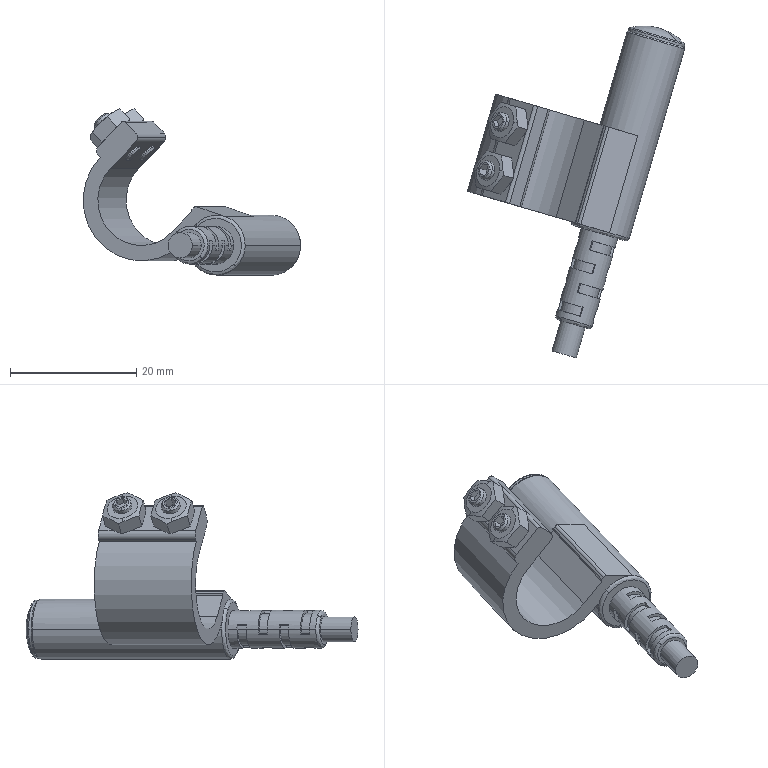Part | SolidWorks | features BaseBody 1 | 1 solid | 143 faces | box 34.458 x 52.569 x 26.335 mm | volume 4644 mm3 | plane 79 | cylinder 38 | cone 16 | spline 10 | commonest cylinder face diameters 5 x12 3 x8 2 x3 0.4 x2 1 x2 4 x2